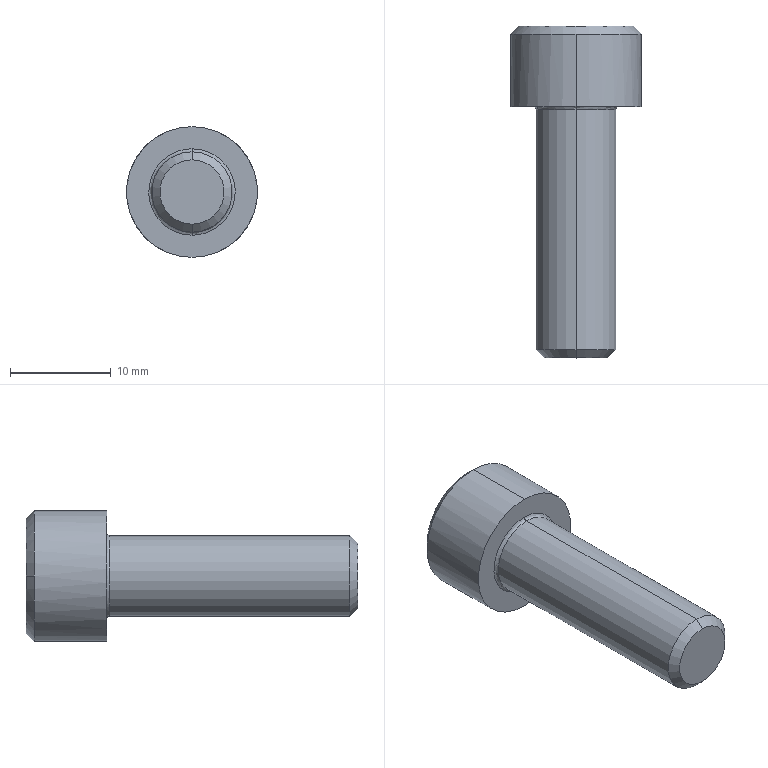Part | STEP file | 1 solid | 20 faces | box 13 x 33 x 13 mm | volume 2112 mm3 | plane 10 | cone 4 | cylinder 4 | spline 2 | commonest cylinder face diameters 8 x2 13 x2